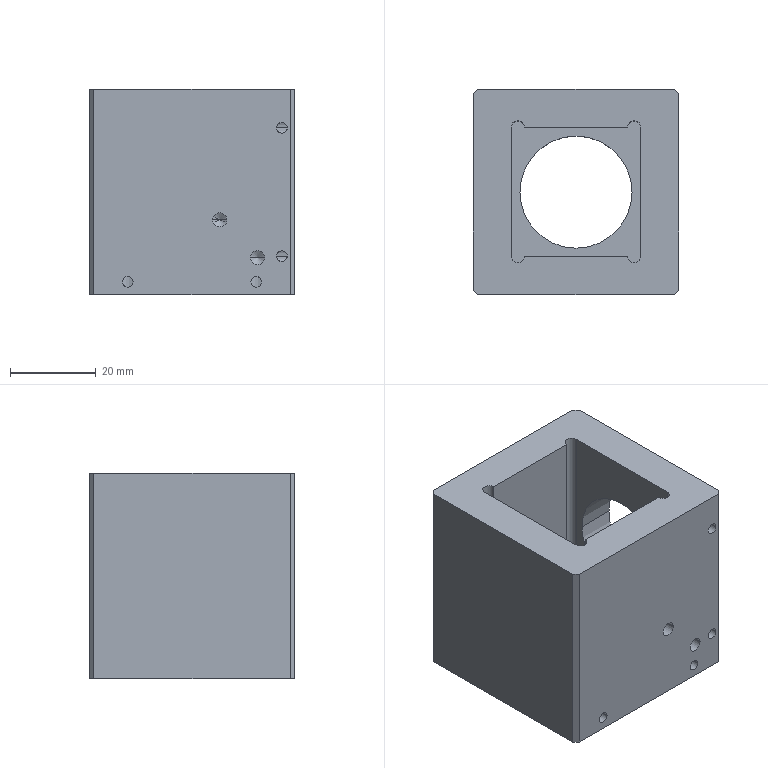NC program | NX | posted with a generic post | part box 48 x 48 x 48 mm
Lines 47 to 927 of 9644:
(ZLEVEL_PROFILE , TOOL : D10)
N80 T15 M6
N82 G54
N84 G17 G0 G90 X-7.746 Y-29.1 B0. C0. S9500 M3
N86 G43 Z30. H15
N88 Z1.5
N90 G94 G1 X-23. Z0.701 F1000.
N92 X-23.554 Z0.672
N94 X-24.963 Y-28.74 Z0.595
N96 X-26.215 Y-27.998 Z0.519
N98 X-26.606 Y-27.606 Z0.49
N100 X-27.606 Y-26.606 Z0.416
N102 X-27.998 Y-26.215 Z0.387
N104 X-28.74 Y-24.963 Z0.311
N106 X-29.1 Y-23.554 Z0.234
N108 Y-23. Z0.205
N110 Y0. Z-1.
N112 Y23. F3200.
N114 G2 X-27.606 Y26.606 R5.1
N116 G1 X-26.606 Y27.606
N118 G2 X-23. Y29.1 R5.1
N120 G1 X23.
N122 G2 X26.606 Y27.606 R5.1
N124 G1 X27.606 Y26.606
N126 G2 X29.1 Y23. R5.1
N128 G1 Y-23.
N130 G2 X27.606 Y-26.606 R5.1
N132 G1 X26.606 Y-27.606
N134 G2 X23. Y-29.1 R5.1
N136 G1 X-23.
N138 G2 X-26.606 Y-27.606 R5.1
N140 G1 X-27.606 Y-26.606
N142 G2 X-29.1 Y-23. R5.1
N144 G1 Y0.
N146 Y22.451 Z-1.392
N148 Y22.839 Z-1.399
N150 X-29.095 Y23.226 Z-1.405
N152 X-29.063 Y23.611 Z-1.412
N154 X-29.002 Y23.993 Z-1.419
N156 X-28.913 Y24.37 Z-1.426
N158 X-28.795 Y24.738 Z-1.432
N160 X-28.649 Y25.097 Z-1.439
N162 X-28.477 Y25.444 Z-1.446
N164 X-28.278 Y25.776 Z-1.453
N166 X-28.056 Y26.092 Z-1.459
N168 X-27.809 Y26.391 Z-1.466
N170 X-27.542 Y26.671 Z-1.473
N172 X-26.994 Y27.218 Z-1.486
N174 X-26.721 Y27.492 Z-1.493
N176 X-26.444 Y27.762 Z-1.5
N178 X-26.148 Y28.012 Z-1.507
N180 X-25.835 Y28.239 Z-1.514
N182 X-25.505 Y28.442 Z-1.52
N184 X-25.161 Y28.619 Z-1.527
N186 X-24.805 Y28.77 Z-1.534
N188 X-24.438 Y28.893 Z-1.541
N190 X-24.063 Y28.988 Z-1.547
N192 X-23.681 Y29.054 Z-1.554
N194 X-23.296 Y29.091 Z-1.561
N196 X-22.909 Y29.1 Z-1.568
N198 X1.865 Z-2.
N200 X23.
N202 G2 X26.606 Y27.606 R5.1
N204 G1 X27.606 Y26.606
N206 G2 X29.1 Y23. R5.1
N208 G1 Y-23.
N210 G2 X27.606 Y-26.606 R5.1
N212 G1 X26.606 Y-27.606
N214 G2 X23. Y-29.1 R5.1
N216 G1 X-23.
N218 G2 X-26.606 Y-27.606 R5.1
N220 G1 X-27.606 Y-26.606
N222 G2 X-29.1 Y-23. R5.1
N224 G1 Y0.
N226 Y22.451 Z-2.392
N228 Y22.839 Z-2.399
N230 X-29.095 Y23.226 Z-2.405
N232 X-29.063 Y23.611 Z-2.412
N234 X-29.002 Y23.993 Z-2.419
N236 X-28.913 Y24.37 Z-2.426
N238 X-28.795 Y24.738 Z-2.432
N240 X-28.649 Y25.097 Z-2.439
N242 X-28.477 Y25.444 Z-2.446
N244 X-28.278 Y25.776 Z-2.453
N246 X-28.056 Y26.092 Z-2.459
N248 X-27.809 Y26.391 Z-2.466
N250 X-27.542 Y26.671 Z-2.473
N252 X-26.994 Y27.218 Z-2.486
N254 X-26.721 Y27.492 Z-2.493
N256 X-26.444 Y27.762 Z-2.5
N258 X-26.148 Y28.012 Z-2.507
N260 X-25.835 Y28.239 Z-2.514
N262 X-25.505 Y28.442 Z-2.52
N264 X-25.161 Y28.619 Z-2.527
N266 X-24.805 Y28.77 Z-2.534
N268 X-24.438 Y28.893 Z-2.541
N270 X-24.063 Y28.988 Z-2.547
N272 X-23.681 Y29.054 Z-2.554
N274 X-23.296 Y29.091 Z-2.561
N276 X-22.909 Y29.1 Z-2.568
N278 X1.865 Z-3.
N280 X23.
N282 G2 X26.606 Y27.606 R5.1
N284 G1 X27.606 Y26.606
N286 G2 X29.1 Y23. R5.1
N288 G1 Y-23.
N290 G2 X27.606 Y-26.606 R5.1
N292 G1 X26.606 Y-27.606
N294 G2 X23. Y-29.1 R5.1
N296 G1 X-23.
N298 G2 X-26.606 Y-27.606 R5.1
N300 G1 X-27.606 Y-26.606
N302 G2 X-29.1 Y-23. R5.1
N304 G1 Y0.
N306 Y22.451 Z-3.392
N308 Y22.839 Z-3.399
N310 X-29.095 Y23.226 Z-3.405
N312 X-29.063 Y23.611 Z-3.412
N314 X-29.002 Y23.993 Z-3.419
N316 X-28.913 Y24.37 Z-3.426
N318 X-28.795 Y24.738 Z-3.432
N320 X-28.649 Y25.097 Z-3.439
N322 X-28.477 Y25.444 Z-3.446
N324 X-28.278 Y25.776 Z-3.453
N326 X-28.056 Y26.092 Z-3.459
N328 X-27.809 Y26.391 Z-3.466
N330 X-27.542 Y26.671 Z-3.473
N332 X-26.994 Y27.218 Z-3.486
N334 X-26.721 Y27.492 Z-3.493
N336 X-26.444 Y27.762 Z-3.5
N338 X-26.148 Y28.012 Z-3.507
N340 X-25.835 Y28.239 Z-3.514
N342 X-25.505 Y28.442 Z-3.52
N344 X-25.161 Y28.619 Z-3.527
N346 X-24.805 Y28.77 Z-3.534
N348 X-24.438 Y28.893 Z-3.541
N350 X-24.063 Y28.988 Z-3.547
N352 X-23.681 Y29.054 Z-3.554
N354 X-23.296 Y29.091 Z-3.561
N356 X-22.909 Y29.1 Z-3.568
N358 X1.865 Z-4.
N360 X23.
N362 G2 X26.606 Y27.606 R5.1
N364 G1 X27.606 Y26.606
N366 G2 X29.1 Y23. R5.1
N368 G1 Y-23.
N370 G2 X27.606 Y-26.606 R5.1
N372 G1 X26.606 Y-27.606
N374 G2 X23. Y-29.1 R5.1
N376 G1 X-23.
N378 G2 X-26.606 Y-27.606 R5.1
N380 G1 X-27.606 Y-26.606
N382 G2 X-29.1 Y-23. R5.1
N384 G1 Y0.
N386 Y22.451 Z-4.392
N388 Y22.839 Z-4.399
N390 X-29.095 Y23.226 Z-4.405
N392 X-29.063 Y23.611 Z-4.412
N394 X-29.002 Y23.993 Z-4.419
N396 X-28.913 Y24.37 Z-4.426
N398 X-28.795 Y24.738 Z-4.432
N400 X-28.649 Y25.097 Z-4.439
N402 X-28.477 Y25.444 Z-4.446
N404 X-28.278 Y25.776 Z-4.453
N406 X-28.056 Y26.092 Z-4.459
N408 X-27.809 Y26.391 Z-4.466
N410 X-27.542 Y26.671 Z-4.473
N412 X-26.994 Y27.218 Z-4.486
N414 X-26.721 Y27.492 Z-4.493
N416 X-26.444 Y27.762 Z-4.5
N418 X-26.148 Y28.012 Z-4.507
N420 X-25.835 Y28.239 Z-4.514
N422 X-25.505 Y28.442 Z-4.52
N424 X-25.161 Y28.619 Z-4.527
N426 X-24.805 Y28.77 Z-4.534
N428 X-24.438 Y28.893 Z-4.541
N430 X-24.063 Y28.988 Z-4.547
N432 X-23.681 Y29.054 Z-4.554
N434 X-23.296 Y29.091 Z-4.561
N436 X-22.909 Y29.1 Z-4.568
N438 X1.865 Z-5.
N440 X23.
N442 G2 X26.606 Y27.606 R5.1
N444 G1 X27.606 Y26.606
N446 G2 X29.1 Y23. R5.1
N448 G1 Y-23.
N450 G2 X27.606 Y-26.606 R5.1
N452 G1 X26.606 Y-27.606
N454 G2 X23. Y-29.1 R5.1
N456 G1 X-23.
N458 G2 X-26.606 Y-27.606 R5.1
N460 G1 X-27.606 Y-26.606
N462 G2 X-29.1 Y-23. R5.1
N464 G1 Y0.
N466 Y22.451 Z-5.392
N468 Y22.839 Z-5.399
N470 X-29.095 Y23.226 Z-5.405
N472 X-29.063 Y23.611 Z-5.412
N474 X-29.002 Y23.993 Z-5.419
N476 X-28.913 Y24.37 Z-5.426
N478 X-28.795 Y24.738 Z-5.432
N480 X-28.649 Y25.097 Z-5.439
N482 X-28.477 Y25.444 Z-5.446
N484 X-28.278 Y25.776 Z-5.453
N486 X-28.056 Y26.092 Z-5.459
N488 X-27.809 Y26.391 Z-5.466
N490 X-27.542 Y26.671 Z-5.473
N492 X-26.994 Y27.218 Z-5.486
N494 X-26.721 Y27.492 Z-5.493
N496 X-26.444 Y27.762 Z-5.5
N498 X-26.148 Y28.012 Z-5.507
N500 X-25.835 Y28.239 Z-5.514
N502 X-25.505 Y28.442 Z-5.52
N504 X-25.161 Y28.619 Z-5.527
N506 X-24.805 Y28.77 Z-5.534
N508 X-24.438 Y28.893 Z-5.541
N510 X-24.063 Y28.988 Z-5.547
N512 X-23.681 Y29.054 Z-5.554
N514 X-23.296 Y29.091 Z-5.561
N516 X-22.909 Y29.1 Z-5.568
N518 X1.865 Z-6.
N520 X23.
N522 G2 X26.606 Y27.606 R5.1
N524 G1 X27.606 Y26.606
N526 G2 X29.1 Y23. R5.1
N528 G1 Y-23.
N530 G2 X27.606 Y-26.606 R5.1
N532 G1 X26.606 Y-27.606
N534 G2 X23. Y-29.1 R5.1
N536 G1 X-23.
N538 G2 X-26.606 Y-27.606 R5.1
N540 G1 X-27.606 Y-26.606
N542 G2 X-29.1 Y-23. R5.1
N544 G1 Y0.
N546 Y22.451 Z-6.392
N548 Y22.839 Z-6.399
N550 X-29.095 Y23.226 Z-6.405
N552 X-29.063 Y23.611 Z-6.412
N554 X-29.002 Y23.993 Z-6.419
N556 X-28.913 Y24.37 Z-6.426
N558 X-28.795 Y24.738 Z-6.432
N560 X-28.649 Y25.097 Z-6.439
N562 X-28.477 Y25.444 Z-6.446
N564 X-28.278 Y25.776 Z-6.453
N566 X-28.056 Y26.092 Z-6.459
N568 X-27.809 Y26.391 Z-6.466
N570 X-27.542 Y26.671 Z-6.473
N572 X-26.994 Y27.218 Z-6.486
N574 X-26.721 Y27.492 Z-6.493
N576 X-26.444 Y27.762 Z-6.5
N578 X-26.148 Y28.012 Z-6.507
N580 X-25.835 Y28.239 Z-6.514
N582 X-25.505 Y28.442 Z-6.52
N584 X-25.161 Y28.619 Z-6.527
N586 X-24.805 Y28.77 Z-6.534
N588 X-24.438 Y28.893 Z-6.541
N590 X-24.063 Y28.988 Z-6.547
N592 X-23.681 Y29.054 Z-6.554
N594 X-23.296 Y29.091 Z-6.561
N596 X-22.909 Y29.1 Z-6.568
N598 X1.865 Z-7.
N600 X23.
N602 G2 X26.606 Y27.606 R5.1
N604 G1 X27.606 Y26.606
N606 G2 X29.1 Y23. R5.1
N608 G1 Y-23.
N610 G2 X27.606 Y-26.606 R5.1
N612 G1 X26.606 Y-27.606
N614 G2 X23. Y-29.1 R5.1
N616 G1 X-23.
N618 G2 X-26.606 Y-27.606 R5.1
N620 G1 X-27.606 Y-26.606
N622 G2 X-29.1 Y-23. R5.1
N624 G1 Y0.
N626 Y22.451 Z-7.392
N628 Y22.839 Z-7.399
N630 X-29.095 Y23.226 Z-7.405
N632 X-29.063 Y23.611 Z-7.412
N634 X-29.002 Y23.993 Z-7.419
N636 X-28.913 Y24.37 Z-7.426
N638 X-28.795 Y24.738 Z-7.432
N640 X-28.649 Y25.097 Z-7.439
N642 X-28.477 Y25.444 Z-7.446
N644 X-28.278 Y25.776 Z-7.453
N646 X-28.056 Y26.092 Z-7.459
N648 X-27.809 Y26.391 Z-7.466
N650 X-27.542 Y26.671 Z-7.473
N652 X-26.994 Y27.218 Z-7.486
N654 X-26.721 Y27.492 Z-7.493
N656 X-26.444 Y27.762 Z-7.5
N658 X-26.148 Y28.012 Z-7.507
N660 X-25.835 Y28.239 Z-7.514
N662 X-25.505 Y28.442 Z-7.52
N664 X-25.161 Y28.619 Z-7.527
N666 X-24.805 Y28.77 Z-7.534
N668 X-24.438 Y28.893 Z-7.541
N670 X-24.063 Y28.988 Z-7.547
N672 X-23.681 Y29.054 Z-7.554
N674 X-23.296 Y29.091 Z-7.561
N676 X-22.909 Y29.1 Z-7.568
N678 X1.865 Z-8.
N680 X23.
N682 G2 X26.606 Y27.606 R5.1
N684 G1 X27.606 Y26.606
N686 G2 X29.1 Y23. R5.1
N688 G1 Y-23.
N690 G2 X27.606 Y-26.606 R5.1
N692 G1 X26.606 Y-27.606
N694 G2 X23. Y-29.1 R5.1
N696 G1 X-23.
N698 G2 X-26.606 Y-27.606 R5.1
N700 G1 X-27.606 Y-26.606
N702 G2 X-29.1 Y-23. R5.1
N704 G1 Y0.
N706 Y22.451 Z-8.392
N708 Y22.839 Z-8.399
N710 X-29.095 Y23.226 Z-8.405
N712 X-29.063 Y23.611 Z-8.412
N714 X-29.002 Y23.993 Z-8.419
N716 X-28.913 Y24.37 Z-8.426
N718 X-28.795 Y24.738 Z-8.432
N720 X-28.649 Y25.097 Z-8.439
N722 X-28.477 Y25.444 Z-8.446
N724 X-28.278 Y25.776 Z-8.453
N726 X-28.056 Y26.092 Z-8.459
N728 X-27.809 Y26.391 Z-8.466
N730 X-27.542 Y26.671 Z-8.473
N732 X-26.994 Y27.218 Z-8.486
N734 X-26.721 Y27.492 Z-8.493
N736 X-26.444 Y27.762 Z-8.5
N738 X-26.148 Y28.012 Z-8.507
N740 X-25.835 Y28.239 Z-8.514
N742 X-25.505 Y28.442 Z-8.52
N744 X-25.161 Y28.619 Z-8.527
N746 X-24.805 Y28.77 Z-8.534
N748 X-24.438 Y28.893 Z-8.541
N750 X-24.063 Y28.988 Z-8.547
N752 X-23.681 Y29.054 Z-8.554
N754 X-23.296 Y29.091 Z-8.561
N756 X-22.909 Y29.1 Z-8.568
N758 X1.865 Z-9.
N760 X23.
N762 G2 X26.606 Y27.606 R5.1
N764 G1 X27.606 Y26.606
N766 G2 X29.1 Y23. R5.1
N768 G1 Y-23.
N770 G2 X27.606 Y-26.606 R5.1
N772 G1 X26.606 Y-27.606
N774 G2 X23. Y-29.1 R5.1
N776 G1 X-23.
N778 G2 X-26.606 Y-27.606 R5.1
N780 G1 X-27.606 Y-26.606
N782 G2 X-29.1 Y-23. R5.1
N784 G1 Y0.
N786 Y22.451 Z-9.392
N788 Y22.839 Z-9.399
N790 X-29.095 Y23.226 Z-9.405
N792 X-29.063 Y23.611 Z-9.412
N794 X-29.002 Y23.993 Z-9.419
N796 X-28.913 Y24.37 Z-9.426
N798 X-28.795 Y24.738 Z-9.432
N800 X-28.649 Y25.097 Z-9.439
N802 X-28.477 Y25.444 Z-9.446
N804 X-28.278 Y25.776 Z-9.453
N806 X-28.056 Y26.092 Z-9.459
N808 X-27.809 Y26.391 Z-9.466
N810 X-27.542 Y26.671 Z-9.473
N812 X-26.994 Y27.218 Z-9.486
N814 X-26.721 Y27.492 Z-9.493
N816 X-26.444 Y27.762 Z-9.5
N818 X-26.148 Y28.012 Z-9.507
N820 X-25.835 Y28.239 Z-9.514
N822 X-25.505 Y28.442 Z-9.52
N824 X-25.161 Y28.619 Z-9.527
N826 X-24.805 Y28.77 Z-9.534
N828 X-24.438 Y28.893 Z-9.541
N830 X-24.063 Y28.988 Z-9.547
N832 X-23.681 Y29.054 Z-9.554
N834 X-23.296 Y29.091 Z-9.561
N836 X-22.909 Y29.1 Z-9.568
N838 X1.865 Z-10.
N840 X23.
N842 G2 X26.606 Y27.606 R5.1
N844 G1 X27.606 Y26.606
N846 G2 X29.1 Y23. R5.1
N848 G1 Y-23.
N850 G2 X27.606 Y-26.606 R5.1
N852 G1 X26.606 Y-27.606
N854 G2 X23. Y-29.1 R5.1
N856 G1 X-23.
N858 G2 X-26.606 Y-27.606 R5.1
N860 G1 X-27.606 Y-26.606
N862 G2 X-29.1 Y-23. R5.1
N864 G1 Y0.
N866 Y22.451 Z-10.392
N868 Y22.839 Z-10.399
N870 X-29.095 Y23.226 Z-10.405
N872 X-29.063 Y23.611 Z-10.412
N874 X-29.002 Y23.993 Z-10.419
N876 X-28.913 Y24.37 Z-10.426
N878 X-28.795 Y24.738 Z-10.432
N880 X-28.649 Y25.097 Z-10.439
N882 X-28.477 Y25.444 Z-10.446
N884 X-28.278 Y25.776 Z-10.453
N886 X-28.056 Y26.092 Z-10.459
N888 X-27.809 Y26.391 Z-10.466
N890 X-27.542 Y26.671 Z-10.473
N892 X-26.994 Y27.218 Z-10.486
N894 X-26.721 Y27.492 Z-10.493
N896 X-26.444 Y27.762 Z-10.5
N898 X-26.148 Y28.012 Z-10.507
N900 X-25.835 Y28.239 Z-10.514
N902 X-25.505 Y28.442 Z-10.52
N904 X-25.161 Y28.619 Z-10.527
N906 X-24.805 Y28.77 Z-10.534
N908 X-24.438 Y28.893 Z-10.541
N910 X-24.063 Y28.988 Z-10.547
N912 X-23.681 Y29.054 Z-10.554
N914 X-23.296 Y29.091 Z-10.561
N916 X-22.909 Y29.1 Z-10.568
N918 X1.865 Z-11.
N920 X23.
N922 G2 X26.606 Y27.606 R5.1
N924 G1 X27.606 Y26.606
N926 G2 X29.1 Y23. R5.1
N928 G1 Y-23.
N930 G2 X27.606 Y-26.606 R5.1
N932 G1 X26.606 Y-27.606
N934 G2 X23. Y-29.1 R5.1
N936 G1 X-23.
N938 G2 X-26.606 Y-27.606 R5.1
N940 G1 X-27.606 Y-26.606
N942 G2 X-29.1 Y-23. R5.1
N944 G1 Y0.
N946 Y22.451 Z-11.392
N948 Y22.839 Z-11.399
N950 X-29.095 Y23.226 Z-11.405
N952 X-29.063 Y23.611 Z-11.412
N954 X-29.002 Y23.993 Z-11.419
N956 X-28.913 Y24.37 Z-11.426
N958 X-28.795 Y24.738 Z-11.432
N960 X-28.649 Y25.097 Z-11.439
N962 X-28.477 Y25.444 Z-11.446
N964 X-28.278 Y25.776 Z-11.453
N966 X-28.056 Y26.092 Z-11.459
N968 X-27.809 Y26.391 Z-11.466
N970 X-27.542 Y26.671 Z-11.473
N972 X-26.994 Y27.218 Z-11.486
N974 X-26.721 Y27.492 Z-11.493
N976 X-26.444 Y27.762 Z-11.5
N978 X-26.148 Y28.012 Z-11.507
N980 X-25.835 Y28.239 Z-11.514
N982 X-25.505 Y28.442 Z-11.52
N984 X-25.161 Y28.619 Z-11.527
N986 X-24.805 Y28.77 Z-11.534
N988 X-24.438 Y28.893 Z-11.541
N990 X-24.063 Y28.988 Z-11.547
N992 X-23.681 Y29.054 Z-11.554
N994 X-23.296 Y29.091 Z-11.561
N996 X-22.909 Y29.1 Z-11.568
N998 X1.865 Z-12.
N1000 X23.
N1002 G2 X26.606 Y27.606 R5.1
N1004 G1 X27.606 Y26.606
N1006 G2 X29.1 Y23. R5.1
N1008 G1 Y-23.
N1010 G2 X27.606 Y-26.606 R5.1
N1012 G1 X26.606 Y-27.606
N1014 G2 X23. Y-29.1 R5.1
N1016 G1 X-23.
N1018 G2 X-26.606 Y-27.606 R5.1
N1020 G1 X-27.606 Y-26.606
N1022 G2 X-29.1 Y-23. R5.1
N1024 G1 Y0.
N1026 Y22.451 Z-12.392
N1028 Y22.839 Z-12.399
N1030 X-29.095 Y23.226 Z-12.405
N1032 X-29.063 Y23.611 Z-12.412
N1034 X-29.002 Y23.993 Z-12.419
N1036 X-28.913 Y24.37 Z-12.426
N1038 X-28.795 Y24.738 Z-12.432
N1040 X-28.649 Y25.097 Z-12.439
N1042 X-28.477 Y25.444 Z-12.446
N1044 X-28.278 Y25.776 Z-12.453
N1046 X-28.056 Y26.092 Z-12.459
N1048 X-27.809 Y26.391 Z-12.466
N1050 X-27.542 Y26.671 Z-12.473
N1052 X-26.994 Y27.218 Z-12.486
N1054 X-26.721 Y27.492 Z-12.493
N1056 X-26.444 Y27.762 Z-12.5
N1058 X-26.148 Y28.012 Z-12.507
N1060 X-25.835 Y28.239 Z-12.514
N1062 X-25.505 Y28.442 Z-12.52
N1064 X-25.161 Y28.619 Z-12.527
N1066 X-24.805 Y28.77 Z-12.534
N1068 X-24.438 Y28.893 Z-12.541
N1070 X-24.063 Y28.988 Z-12.547
N1072 X-23.681 Y29.054 Z-12.554
N1074 X-23.296 Y29.091 Z-12.561
N1076 X-22.909 Y29.1 Z-12.568
N1078 X1.865 Z-13.
N1080 X23.
N1082 G2 X26.606 Y27.606 R5.1
N1084 G1 X27.606 Y26.606
N1086 G2 X29.1 Y23. R5.1
N1088 G1 Y-23.
N1090 G2 X27.606 Y-26.606 R5.1
N1092 G1 X26.606 Y-27.606
N1094 G2 X23. Y-29.1 R5.1
N1096 G1 X-23.
N1098 G2 X-26.606 Y-27.606 R5.1
N1100 G1 X-27.606 Y-26.606
N1102 G2 X-29.1 Y-23. R5.1
N1104 G1 Y0.
N1106 Y22.451 Z-13.392
N1108 Y22.839 Z-13.399
N1110 X-29.095 Y23.226 Z-13.405
N1112 X-29.063 Y23.611 Z-13.412
N1114 X-29.002 Y23.993 Z-13.419
N1116 X-28.913 Y24.37 Z-13.426
N1118 X-28.795 Y24.738 Z-13.432
N1120 X-28.649 Y25.097 Z-13.439
N1122 X-28.477 Y25.444 Z-13.446
N1124 X-28.278 Y25.776 Z-13.453
N1126 X-28.056 Y26.092 Z-13.459
N1128 X-27.809 Y26.391 Z-13.466
N1130 X-27.542 Y26.671 Z-13.473
N1132 X-26.994 Y27.218 Z-13.486
N1134 X-26.721 Y27.492 Z-13.493
N1136 X-26.444 Y27.762 Z-13.5
N1138 X-26.148 Y28.012 Z-13.507
N1140 X-25.835 Y28.239 Z-13.514
N1142 X-25.505 Y28.442 Z-13.52
N1144 X-25.161 Y28.619 Z-13.527
N1146 X-24.805 Y28.77 Z-13.534
N1148 X-24.438 Y28.893 Z-13.541
N1150 X-24.063 Y28.988 Z-13.547
N1152 X-23.681 Y29.054 Z-13.554
N1154 X-23.296 Y29.091 Z-13.561
N1156 X-22.909 Y29.1 Z-13.568
N1158 X1.865 Z-14.
N1160 X23.
N1162 G2 X26.606 Y27.606 R5.1
N1164 G1 X27.606 Y26.606
N1166 G2 X29.1 Y23. R5.1
N1168 G1 Y-23.
N1170 G2 X27.606 Y-26.606 R5.1
N1172 G1 X26.606 Y-27.606
N1174 G2 X23. Y-29.1 R5.1
N1176 G1 X-23.
N1178 G2 X-26.606 Y-27.606 R5.1
N1180 G1 X-27.606 Y-26.606
N1182 G2 X-29.1 Y-23. R5.1
N1184 G1 Y0.
N1186 Y22.451 Z-14.392
N1188 Y22.839 Z-14.399
N1190 X-29.095 Y23.226 Z-14.405
N1192 X-29.063 Y23.611 Z-14.412
N1194 X-29.002 Y23.993 Z-14.419
N1196 X-28.913 Y24.37 Z-14.426
N1198 X-28.795 Y24.738 Z-14.432
N1200 X-28.649 Y25.097 Z-14.439
N1202 X-28.477 Y25.444 Z-14.446
N1204 X-28.278 Y25.776 Z-14.453
N1206 X-28.056 Y26.092 Z-14.459
N1208 X-27.809 Y26.391 Z-14.466
N1210 X-27.542 Y26.671 Z-14.473
N1212 X-26.994 Y27.218 Z-14.486
N1214 X-26.721 Y27.492 Z-14.493
N1216 X-26.444 Y27.762 Z-14.5
N1218 X-26.148 Y28.012 Z-14.507
N1220 X-25.835 Y28.239 Z-14.514
N1222 X-25.505 Y28.442 Z-14.52
N1224 X-25.161 Y28.619 Z-14.527
N1226 X-24.805 Y28.77 Z-14.534
N1228 X-24.438 Y28.893 Z-14.541
N1230 X-24.063 Y28.988 Z-14.547
N1232 X-23.681 Y29.054 Z-14.554
N1234 X-23.296 Y29.091 Z-14.561
N1236 X-22.909 Y29.1 Z-14.568
N1238 X1.865 Z-15.
N1240 X23.
N1242 G2 X26.606 Y27.606 R5.1
N1244 G1 X27.606 Y26.606
N1246 G2 X29.1 Y23. R5.1
N1248 G1 Y-23.
N1250 G2 X27.606 Y-26.606 R5.1
N1252 G1 X26.606 Y-27.606
N1254 G2 X23. Y-29.1 R5.1
N1256 G1 X-23.
N1258 G2 X-26.606 Y-27.606 R5.1
N1260 G1 X-27.606 Y-26.606
N1262 G2 X-29.1 Y-23. R5.1
N1264 G1 Y0.
N1266 Y22.451 Z-15.392
N1268 Y22.839 Z-15.399
N1270 X-29.095 Y23.226 Z-15.405
N1272 X-29.063 Y23.611 Z-15.412
N1274 X-29.002 Y23.993 Z-15.419
N1276 X-28.913 Y24.37 Z-15.426
N1278 X-28.795 Y24.738 Z-15.432
N1280 X-28.649 Y25.097 Z-15.439
N1282 X-28.477 Y25.444 Z-15.446
N1284 X-28.278 Y25.776 Z-15.453
N1286 X-28.056 Y26.092 Z-15.459
N1288 X-27.809 Y26.391 Z-15.466
N1290 X-27.542 Y26.671 Z-15.473
N1292 X-26.994 Y27.218 Z-15.486
N1294 X-26.721 Y27.492 Z-15.493
N1296 X-26.444 Y27.762 Z-15.5
N1298 X-26.148 Y28.012 Z-15.507
N1300 X-25.835 Y28.239 Z-15.514
N1302 X-25.505 Y28.442 Z-15.52
N1304 X-25.161 Y28.619 Z-15.527
N1306 X-24.805 Y28.77 Z-15.534
N1308 X-24.438 Y28.893 Z-15.541
N1310 X-24.063 Y28.988 Z-15.547
N1312 X-23.681 Y29.054 Z-15.554
N1314 X-23.296 Y29.091 Z-15.561
N1316 X-22.909 Y29.1 Z-15.568
N1318 X1.865 Z-16.
N1320 X23.
N1322 G2 X26.606 Y27.606 R5.1
N1324 G1 X27.606 Y26.606
N1326 G2 X29.1 Y23. R5.1
N1328 G1 Y-23.
N1330 G2 X27.606 Y-26.606 R5.1
N1332 G1 X26.606 Y-27.606
N1334 G2 X23. Y-29.1 R5.1
N1336 G1 X-23.
N1338 G2 X-26.606 Y-27.606 R5.1
N1340 G1 X-27.606 Y-26.606
N1342 G2 X-29.1 Y-23. R5.1
N1344 G1 Y0.
N1346 Y22.451 Z-16.392
N1348 Y22.839 Z-16.399
N1350 X-29.095 Y23.226 Z-16.405
N1352 X-29.063 Y23.611 Z-16.412
N1354 X-29.002 Y23.993 Z-16.419
N1356 X-28.913 Y24.37 Z-16.426
N1358 X-28.795 Y24.738 Z-16.432
N1360 X-28.649 Y25.097 Z-16.439
N1362 X-28.477 Y25.444 Z-16.446
N1364 X-28.278 Y25.776 Z-16.453
N1366 X-28.056 Y26.092 Z-16.459
N1368 X-27.809 Y26.391 Z-16.466
N1370 X-27.542 Y26.671 Z-16.473
N1372 X-26.994 Y27.218 Z-16.486
N1374 X-26.721 Y27.492 Z-16.493
N1376 X-26.444 Y27.762 Z-16.5
N1378 X-26.148 Y28.012 Z-16.507
N1380 X-25.835 Y28.239 Z-16.514
N1382 X-25.505 Y28.442 Z-16.52
N1384 X-25.161 Y28.619 Z-16.527
N1386 X-24.805 Y28.77 Z-16.534
N1388 X-24.438 Y28.893 Z-16.541
N1390 X-24.063 Y28.988 Z-16.547
N1392 X-23.681 Y29.054 Z-16.554
N1394 X-23.296 Y29.091 Z-16.561
N1396 X-22.909 Y29.1 Z-16.568
N1398 X1.865 Z-17.
N1400 X23.
N1402 G2 X26.606 Y27.606 R5.1
N1404 G1 X27.606 Y26.606
N1406 G2 X29.1 Y23. R5.1
N1408 G1 Y-23.
N1410 G2 X27.606 Y-26.606 R5.1
N1412 G1 X26.606 Y-27.606
N1414 G2 X23. Y-29.1 R5.1
N1416 G1 X-23.
N1418 G2 X-26.606 Y-27.606 R5.1
N1420 G1 X-27.606 Y-26.606
N1422 G2 X-29.1 Y-23. R5.1
N1424 G1 Y0.
N1426 Y22.451 Z-17.392
N1428 Y22.839 Z-17.399
N1430 X-29.095 Y23.226 Z-17.405
N1432 X-29.063 Y23.611 Z-17.412
N1434 X-29.002 Y23.993 Z-17.419
N1436 X-28.913 Y24.37 Z-17.426
N1438 X-28.795 Y24.738 Z-17.432
N1440 X-28.649 Y25.097 Z-17.439
N1442 X-28.477 Y25.444 Z-17.446
N1444 X-28.278 Y25.776 Z-17.453
N1446 X-28.056 Y26.092 Z-17.459
N1448 X-27.809 Y26.391 Z-17.466
N1450 X-27.542 Y26.671 Z-17.473
N1452 X-26.994 Y27.218 Z-17.486
N1454 X-26.721 Y27.492 Z-17.493
N1456 X-26.444 Y27.762 Z-17.5
N1458 X-26.148 Y28.012 Z-17.507
N1460 X-25.835 Y28.239 Z-17.514
N1462 X-25.505 Y28.442 Z-17.52
N1464 X-25.161 Y28.619 Z-17.527
N1466 X-24.805 Y28.77 Z-17.534
N1468 X-24.438 Y28.893 Z-17.541
N1470 X-24.063 Y28.988 Z-17.547
N1472 X-23.681 Y29.054 Z-17.554
N1474 X-23.296 Y29.091 Z-17.561
N1476 X-22.909 Y29.1 Z-17.568
N1478 X1.865 Z-18.
N1480 X23.
N1482 G2 X26.606 Y27.606 R5.1
N1484 G1 X27.606 Y26.606
N1486 G2 X29.1 Y23. R5.1
N1488 G1 Y-23.
N1490 G2 X27.606 Y-26.606 R5.1
N1492 G1 X26.606 Y-27.606
N1494 G2 X23. Y-29.1 R5.1
N1496 G1 X-23.
N1498 G2 X-26.606 Y-27.606 R5.1
N1500 G1 X-27.606 Y-26.606
N1502 G2 X-29.1 Y-23. R5.1
N1504 G1 Y0.
N1506 Y22.451 Z-18.392
N1508 Y22.839 Z-18.399
N1510 X-29.095 Y23.226 Z-18.405
N1512 X-29.063 Y23.611 Z-18.412
N1514 X-29.002 Y23.993 Z-18.419
N1516 X-28.913 Y24.37 Z-18.426
N1518 X-28.795 Y24.738 Z-18.432
N1520 X-28.649 Y25.097 Z-18.439
N1522 X-28.477 Y25.444 Z-18.446
N1524 X-28.278 Y25.776 Z-18.453
N1526 X-28.056 Y26.092 Z-18.459
N1528 X-27.809 Y26.391 Z-18.466
N1530 X-27.542 Y26.671 Z-18.473
N1532 X-26.994 Y27.218 Z-18.486
N1534 X-26.721 Y27.492 Z-18.493
N1536 X-26.444 Y27.762 Z-18.5
N1538 X-26.148 Y28.012 Z-18.507
N1540 X-25.835 Y28.239 Z-18.514
N1542 X-25.505 Y28.442 Z-18.52
N1544 X-25.161 Y28.619 Z-18.527
N1546 X-24.805 Y28.77 Z-18.534
N1548 X-24.438 Y28.893 Z-18.541
N1550 X-24.063 Y28.988 Z-18.547
N1552 X-23.681 Y29.054 Z-18.554
N1554 X-23.296 Y29.091 Z-18.561
N1556 X-22.909 Y29.1 Z-18.568
N1558 X1.865 Z-19.
N1560 X23.
N1562 G2 X26.606 Y27.606 R5.1
N1564 G1 X27.606 Y26.606
N1566 G2 X29.1 Y23. R5.1
N1568 G1 Y-23.
N1570 G2 X27.606 Y-26.606 R5.1
N1572 G1 X26.606 Y-27.606
N1574 G2 X23. Y-29.1 R5.1
N1576 G1 X-23.
N1578 G2 X-26.606 Y-27.606 R5.1
N1580 G1 X-27.606 Y-26.606
N1582 G2 X-29.1 Y-23. R5.1
N1584 G1 Y0.
N1586 Y22.451 Z-19.392
N1588 Y22.839 Z-19.399
N1590 X-29.095 Y23.226 Z-19.405
N1592 X-29.063 Y23.611 Z-19.412
N1594 X-29.002 Y23.993 Z-19.419
N1596 X-28.913 Y24.37 Z-19.426
N1598 X-28.795 Y24.738 Z-19.432
N1600 X-28.649 Y25.097 Z-19.439
N1602 X-28.477 Y25.444 Z-19.446
N1604 X-28.278 Y25.776 Z-19.453
N1606 X-28.056 Y26.092 Z-19.459
N1608 X-27.809 Y26.391 Z-19.466
N1610 X-27.542 Y26.671 Z-19.473
N1612 X-26.994 Y27.218 Z-19.486
N1614 X-26.721 Y27.492 Z-19.493
N1616 X-26.444 Y27.762 Z-19.5
N1618 X-26.148 Y28.012 Z-19.507
N1620 X-25.835 Y28.239 Z-19.514
N1622 X-25.505 Y28.442 Z-19.52
N1624 X-25.161 Y28.619 Z-19.527
N1626 X-24.805 Y28.77 Z-19.534
N1628 X-24.438 Y28.893 Z-19.541
N1630 X-24.063 Y28.988 Z-19.547
N1632 X-23.681 Y29.054 Z-19.554
N1634 X-23.296 Y29.091 Z-19.561
N1636 X-22.909 Y29.1 Z-19.568
N1638 X1.865 Z-20.
N1640 X23.
N1642 G2 X26.606 Y27.606 R5.1
N1644 G1 X27.606 Y26.606
N1646 G2 X29.1 Y23. R5.1
N1648 G1 Y-23.
N1650 G2 X27.606 Y-26.606 R5.1
N1652 G1 X26.606 Y-27.606
N1654 G2 X23. Y-29.1 R5.1
N1656 G1 X-23.
N1658 G2 X-26.606 Y-27.606 R5.1
N1660 G1 X-27.606 Y-26.606
N1662 G2 X-29.1 Y-23. R5.1
N1664 G1 Y0.
N1666 Y22.451 Z-20.392
N1668 Y22.839 Z-20.399
N1670 X-29.095 Y23.226 Z-20.405
N1672 X-29.063 Y23.611 Z-20.412
N1674 X-29.002 Y23.993 Z-20.419
N1676 X-28.913 Y24.37 Z-20.426
N1678 X-28.795 Y24.738 Z-20.432
N1680 X-28.649 Y25.097 Z-20.439
N1682 X-28.477 Y25.444 Z-20.446
N1684 X-28.278 Y25.776 Z-20.453
N1686 X-28.056 Y26.092 Z-20.459
N1688 X-27.809 Y26.391 Z-20.466
N1690 X-27.542 Y26.671 Z-20.473
N1692 X-26.994 Y27.218 Z-20.486
N1694 X-26.721 Y27.492 Z-20.493
N1696 X-26.444 Y27.762 Z-20.5
N1698 X-26.148 Y28.012 Z-20.507
N1700 X-25.835 Y28.239 Z-20.514
N1702 X-25.505 Y28.442 Z-20.52
N1704 X-25.161 Y28.619 Z-20.527
N1706 X-24.805 Y28.77 Z-20.534
N1708 X-24.438 Y28.893 Z-20.541
N1710 X-24.063 Y28.988 Z-20.547
N1712 X-23.681 Y29.054 Z-20.554
N1714 X-23.296 Y29.091 Z-20.561
N1716 X-22.909 Y29.1 Z-20.568
N1718 X1.865 Z-21.
N1720 X23.
N1722 G2 X26.606 Y27.606 R5.1
N1724 G1 X27.606 Y26.606
N1726 G2 X29.1 Y23. R5.1
N1728 G1 Y-23.
N1730 G2 X27.606 Y-26.606 R5.1
N1732 G1 X26.606 Y-27.606
N1734 G2 X23. Y-29.1 R5.1
N1736 G1 X-23.
N1738 G2 X-26.606 Y-27.606 R5.1
N1740 G1 X-27.606 Y-26.606
N1742 G2 X-29.1 Y-23. R5.1
N1744 G1 Y0.
N1746 Y22.451 Z-21.392
N1748 Y22.839 Z-21.399
N1750 X-29.095 Y23.226 Z-21.405
N1752 X-29.063 Y23.611 Z-21.412
N1754 X-29.002 Y23.993 Z-21.419
N1756 X-28.913 Y24.37 Z-21.426
N1758 X-28.795 Y24.738 Z-21.432
N1760 X-28.649 Y25.097 Z-21.439
N1762 X-28.477 Y25.444 Z-21.446
N1764 X-28.278 Y25.776 Z-21.453
N1766 X-28.056 Y26.092 Z-21.459
N1768 X-27.809 Y26.391 Z-21.466
N1770 X-27.542 Y26.671 Z-21.473
N1772 X-26.994 Y27.218 Z-21.486
N1774 X-26.721 Y27.492 Z-21.493
N1776 X-26.444 Y27.762 Z-21.5
N1778 X-26.148 Y28.012 Z-21.507
N1780 X-25.835 Y28.239 Z-21.514
N1782 X-25.505 Y28.442 Z-21.52
N1784 X-25.161 Y28.619 Z-21.527
N1786 X-24.805 Y28.77 Z-21.534
N1788 X-24.438 Y28.893 Z-21.541
N1790 X-24.063 Y28.988 Z-21.547
N1792 X-23.681 Y29.054 Z-21.554
N1794 X-23.296 Y29.091 Z-21.561
N1796 X-22.909 Y29.1 Z-21.568
N1798 X1.865 Z-22.
N1800 X23.
N1802 G2 X26.606 Y27.606 R5.1
N1804 G1 X27.606 Y26.606
N1806 G2 X29.1 Y23. R5.1
N1808 G1 Y-23.
N1810 G2 X27.606 Y-26.606 R5.1
N1812 G1 X26.606 Y-27.606
N1814 G2 X23. Y-29.1 R5.1
N1816 G1 X-23.
N1818 G2 X-26.606 Y-27.606 R5.1
N1820 G1 X-27.606 Y-26.606
N1822 G2 X-29.1 Y-23. R5.1
N1824 G1 Y0.
N1826 Y22.451 Z-22.392
N1828 Y22.839 Z-22.399
N1830 X-29.095 Y23.226 Z-22.405
N1832 X-29.063 Y23.611 Z-22.412
N1834 X-29.002 Y23.993 Z-22.419